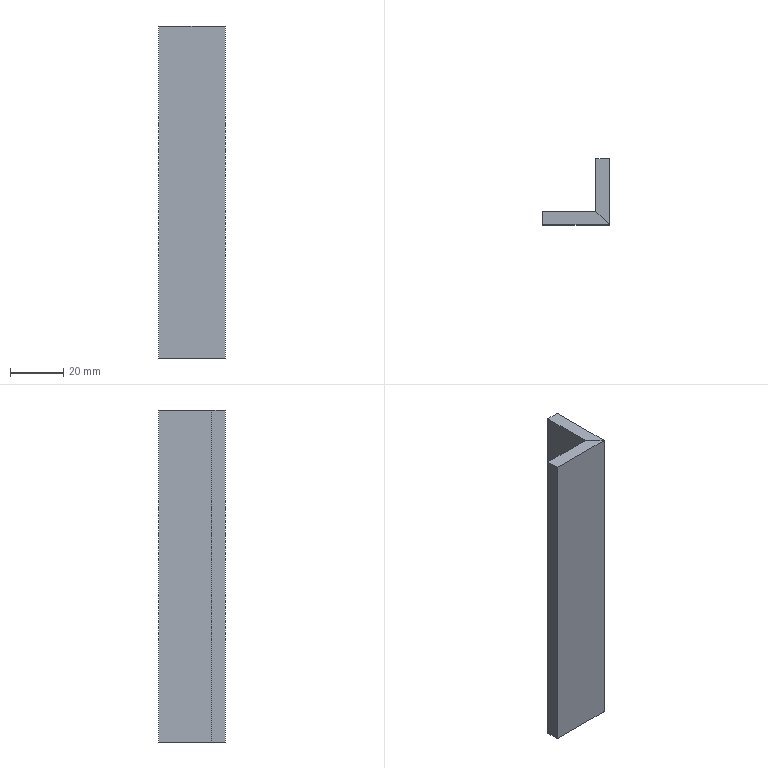Part | NX | features BREP 1 | 1 solid | 10 faces | box 25 x 25 x 125 mm | volume 28125 mm3 | plane 10
STEP:
#1=CARTESIAN_POINT('',(689.674,-673.,218.142));
#2=VERTEX_POINT('',#1);
#3=CARTESIAN_POINT('',(694.674,-673.,218.142));
#4=VERTEX_POINT('',#3);
#5=CARTESIAN_POINT('',(692.174,-673.,218.142));
#6=DIRECTION('',(1.,0.,0.));
#7=VECTOR('',#6,1000.);
#8=LINE('',#5,#7);
#9=EDGE_CURVE('',#2,#4,#8,.T.);
#10=ORIENTED_EDGE('',*,*,#9,.F.);
#11=CARTESIAN_POINT('',(689.674,-693.,218.142));
#12=VERTEX_POINT('',#11);
#13=CARTESIAN_POINT('',(689.674,-683.,218.142));
#14=DIRECTION('',(0.,1.,0.));
#15=VECTOR('',#14,1000.);
#16=LINE('',#13,#15);
#17=EDGE_CURVE('',#12,#2,#16,.T.);
#18=ORIENTED_EDGE('',*,*,#17,.F.);
#19=CARTESIAN_POINT('',(694.674,-698.,218.142));
#20=VERTEX_POINT('',#19);
#21=CARTESIAN_POINT('',(692.174,-695.5,218.142));
#22=DIRECTION('',(-0.7071,0.7071,0.));
#23=VECTOR('',#22,1000.);
#24=LINE('',#21,#23);
#25=EDGE_CURVE('',#20,#12,#24,.T.);
#26=ORIENTED_EDGE('',*,*,#25,.F.);
#27=CARTESIAN_POINT('',(694.674,-685.5,218.142));
#28=DIRECTION('',(0.,1.,0.));
#29=VECTOR('',#28,1000.);
#30=LINE('',#27,#29);
#31=EDGE_CURVE('',#20,#4,#30,.T.);
#32=ORIENTED_EDGE('',*,*,#31,.T.);
#33=EDGE_LOOP('',(#10,#18,#26,#32));
#34=FACE_BOUND('',#33,.T.);
#35=CARTESIAN_POINT('',(694.674,-685.5,218.142));
#36=DIRECTION('',(0.,0.,-1.));
#37=DIRECTION('',(1.,0.,0.));
#38=AXIS2_PLACEMENT_3D('',#35,#36,#37);
#39=PLANE('',#38);
#40=ADVANCED_FACE('',(#34),#39,.F.);
#41=CARTESIAN_POINT('',(689.674,-673.,93.142));
#42=VERTEX_POINT('',#41);
#43=CARTESIAN_POINT('',(694.674,-673.,93.142));
#44=VERTEX_POINT('',#43);
#45=CARTESIAN_POINT('',(692.174,-673.,93.142));
#46=DIRECTION('',(1.,0.,0.));
#47=VECTOR('',#46,1000.);
#48=LINE('',#45,#47);
#49=EDGE_CURVE('',#42,#44,#48,.T.);
#50=ORIENTED_EDGE('',*,*,#49,.F.);
#51=CARTESIAN_POINT('',(689.674,-673.,155.642));
#52=DIRECTION('',(0.,0.,1.));
#53=VECTOR('',#52,1000.);
#54=LINE('',#51,#53);
#55=EDGE_CURVE('',#42,#2,#54,.T.);
#56=ORIENTED_EDGE('',*,*,#55,.T.);
#57=ORIENTED_EDGE('',*,*,#9,.T.);
#58=CARTESIAN_POINT('',(694.674,-673.,155.642));
#59=DIRECTION('',(0.,0.,1.));
#60=VECTOR('',#59,1000.);
#61=LINE('',#58,#60);
#62=EDGE_CURVE('',#44,#4,#61,.T.);
#63=ORIENTED_EDGE('',*,*,#62,.F.);
#64=EDGE_LOOP('',(#50,#56,#57,#63));
#65=FACE_BOUND('',#64,.T.);
#66=CARTESIAN_POINT('',(694.674,-673.,155.642));
#67=DIRECTION('',(0.,1.,0.));
#68=DIRECTION('',(1.,0.,0.));
#69=AXIS2_PLACEMENT_3D('',#66,#67,#68);
#70=PLANE('',#69);
#71=ADVANCED_FACE('',(#65),#70,.T.);
#72=ORIENTED_EDGE('',*,*,#31,.F.);
#73=CARTESIAN_POINT('',(694.674,-698.,93.142));
#74=VERTEX_POINT('',#73);
#75=CARTESIAN_POINT('',(694.674,-698.,155.642));
#76=DIRECTION('',(0.,0.,1.));
#77=VECTOR('',#76,1000.);
#78=LINE('',#75,#77);
#79=EDGE_CURVE('',#74,#20,#78,.T.);
#80=ORIENTED_EDGE('',*,*,#79,.F.);
#81=CARTESIAN_POINT('',(694.674,-685.5,93.142));
#82=DIRECTION('',(0.,-1.,0.));
#83=VECTOR('',#82,1000.);
#84=LINE('',#81,#83);
#85=EDGE_CURVE('',#44,#74,#84,.T.);
#86=ORIENTED_EDGE('',*,*,#85,.F.);
#87=ORIENTED_EDGE('',*,*,#62,.T.);
#88=EDGE_LOOP('',(#72,#80,#86,#87));
#89=FACE_BOUND('',#88,.T.);
#90=CARTESIAN_POINT('',(694.674,-700.,74.));
#91=DIRECTION('',(-1.,0.,0.));
#92=DIRECTION('',(0.,0.,1.));
#93=AXIS2_PLACEMENT_3D('',#90,#91,#92);
#94=PLANE('',#93);
#95=ADVANCED_FACE('',(#89),#94,.F.);
#96=ORIENTED_EDGE('',*,*,#55,.F.);
#97=CARTESIAN_POINT('',(689.674,-693.,93.142));
#98=VERTEX_POINT('',#97);
#99=CARTESIAN_POINT('',(689.674,-683.,93.142));
#100=DIRECTION('',(0.,-1.,0.));
#101=VECTOR('',#100,1000.);
#102=LINE('',#99,#101);
#103=EDGE_CURVE('',#42,#98,#102,.T.);
#104=ORIENTED_EDGE('',*,*,#103,.T.);
#105=CARTESIAN_POINT('',(689.674,-693.,155.642));
#106=DIRECTION('',(0.,0.,1.));
#107=VECTOR('',#106,1000.);
#108=LINE('',#105,#107);
#109=EDGE_CURVE('',#98,#12,#108,.T.);
#110=ORIENTED_EDGE('',*,*,#109,.T.);
#111=ORIENTED_EDGE('',*,*,#17,.T.);
#112=EDGE_LOOP('',(#96,#104,#110,#111));
#113=FACE_BOUND('',#112,.T.);
#114=CARTESIAN_POINT('',(689.674,-700.,74.));
#115=DIRECTION('',(-1.,0.,0.));
#116=DIRECTION('',(0.,0.,1.));
#117=AXIS2_PLACEMENT_3D('',#114,#115,#116);
#118=PLANE('',#117);
#119=ADVANCED_FACE('',(#113),#118,.T.);
#120=CARTESIAN_POINT('',(669.674,-698.,218.142));
#121=VERTEX_POINT('',#120);
#122=CARTESIAN_POINT('',(682.174,-698.,218.142));
#123=DIRECTION('',(-1.,0.,0.));
#124=VECTOR('',#123,1000.);
#125=LINE('',#122,#124);
#126=EDGE_CURVE('',#20,#121,#125,.T.);
#127=ORIENTED_EDGE('',*,*,#126,.F.);
#128=ORIENTED_EDGE('',*,*,#25,.T.);
#129=CARTESIAN_POINT('',(669.674,-693.,218.142));
#130=VERTEX_POINT('',#129);
#131=CARTESIAN_POINT('',(679.674,-693.,218.142));
#132=DIRECTION('',(-1.,0.,0.));
#133=VECTOR('',#132,1000.);
#134=LINE('',#131,#133);
#135=EDGE_CURVE('',#12,#130,#134,.T.);
#136=ORIENTED_EDGE('',*,*,#135,.T.);
#137=CARTESIAN_POINT('',(669.674,-695.5,218.142));
#138=DIRECTION('',(0.,-1.,0.));
#139=VECTOR('',#138,1000.);
#140=LINE('',#137,#139);
#141=EDGE_CURVE('',#130,#121,#140,.T.);
#142=ORIENTED_EDGE('',*,*,#141,.T.);
#143=EDGE_LOOP('',(#127,#128,#136,#142));
#144=FACE_BOUND('',#143,.T.);
#145=CARTESIAN_POINT('',(694.674,-698.,218.142));
#146=DIRECTION('',(0.,0.,1.));
#147=DIRECTION('',(-1.,0.,0.));
#148=AXIS2_PLACEMENT_3D('',#145,#146,#147);
#149=PLANE('',#148);
#150=ADVANCED_FACE('',(#144),#149,.T.);
#151=CARTESIAN_POINT('',(669.674,-698.,93.142));
#152=VERTEX_POINT('',#151);
#153=CARTESIAN_POINT('',(682.174,-698.,93.142));
#154=DIRECTION('',(-1.,0.,0.));
#155=VECTOR('',#154,1000.);
#156=LINE('',#153,#155);
#157=EDGE_CURVE('',#74,#152,#156,.T.);
#158=ORIENTED_EDGE('',*,*,#157,.F.);
#159=ORIENTED_EDGE('',*,*,#79,.T.);
#160=ORIENTED_EDGE('',*,*,#126,.T.);
#161=CARTESIAN_POINT('',(669.674,-698.,155.642));
#162=DIRECTION('',(0.,0.,1.));
#163=VECTOR('',#162,1000.);
#164=LINE('',#161,#163);
#165=EDGE_CURVE('',#152,#121,#164,.T.);
#166=ORIENTED_EDGE('',*,*,#165,.F.);
#167=EDGE_LOOP('',(#158,#159,#160,#166));
#168=FACE_BOUND('',#167,.T.);
#169=CARTESIAN_POINT('',(694.674,-698.,93.142));
#170=DIRECTION('',(0.,-1.,0.));
#171=DIRECTION('',(0.,0.,1.));
#172=AXIS2_PLACEMENT_3D('',#169,#170,#171);
#173=PLANE('',#172);
#174=ADVANCED_FACE('',(#168),#173,.T.);
#175=ORIENTED_EDGE('',*,*,#85,.T.);
#176=CARTESIAN_POINT('',(692.174,-695.5,93.142));
#177=DIRECTION('',(-0.7071,0.7071,0.));
#178=VECTOR('',#177,1000.);
#179=LINE('',#176,#178);
#180=EDGE_CURVE('',#74,#98,#179,.T.);
#181=ORIENTED_EDGE('',*,*,#180,.T.);
#182=ORIENTED_EDGE('',*,*,#103,.F.);
#183=ORIENTED_EDGE('',*,*,#49,.T.);
#184=EDGE_LOOP('',(#175,#181,#182,#183));
#185=FACE_BOUND('',#184,.T.);
#186=CARTESIAN_POINT('',(694.674,-685.5,93.142));
#187=DIRECTION('',(0.,0.,-1.));
#188=DIRECTION('',(1.,0.,0.));
#189=AXIS2_PLACEMENT_3D('',#186,#187,#188);
#190=PLANE('',#189);
#191=ADVANCED_FACE('',(#185),#190,.T.);
#192=CARTESIAN_POINT('',(669.674,-693.,93.142));
#193=VERTEX_POINT('',#192);
#194=CARTESIAN_POINT('',(669.674,-693.,155.642));
#195=DIRECTION('',(0.,0.,1.));
#196=VECTOR('',#195,1000.);
#197=LINE('',#194,#196);
#198=EDGE_CURVE('',#193,#130,#197,.T.);
#199=ORIENTED_EDGE('',*,*,#198,.T.);
#200=ORIENTED_EDGE('',*,*,#135,.F.);
#201=ORIENTED_EDGE('',*,*,#109,.F.);
#202=CARTESIAN_POINT('',(679.674,-693.,93.142));
#203=DIRECTION('',(-1.,0.,0.));
#204=VECTOR('',#203,1000.);
#205=LINE('',#202,#204);
#206=EDGE_CURVE('',#98,#193,#205,.T.);
#207=ORIENTED_EDGE('',*,*,#206,.T.);
#208=EDGE_LOOP('',(#199,#200,#201,#207));
#209=FACE_BOUND('',#208,.T.);
#210=CARTESIAN_POINT('',(689.674,-693.,93.142));
#211=DIRECTION('',(0.,-1.,0.));
#212=DIRECTION('',(0.,0.,1.));
#213=AXIS2_PLACEMENT_3D('',#210,#211,#212);
#214=PLANE('',#213);
#215=ADVANCED_FACE('',(#209),#214,.F.);
#216=ORIENTED_EDGE('',*,*,#165,.T.);
#217=ORIENTED_EDGE('',*,*,#141,.F.);
#218=ORIENTED_EDGE('',*,*,#198,.F.);
#219=CARTESIAN_POINT('',(669.674,-695.5,93.142));
#220=DIRECTION('',(0.,-1.,0.));
#221=VECTOR('',#220,1000.);
#222=LINE('',#219,#221);
#223=EDGE_CURVE('',#193,#152,#222,.T.);
#224=ORIENTED_EDGE('',*,*,#223,.T.);
#225=EDGE_LOOP('',(#216,#217,#218,#224));
#226=FACE_BOUND('',#225,.T.);
#227=CARTESIAN_POINT('',(669.674,-698.,93.142));
#228=DIRECTION('',(1.,0.,0.));
#229=DIRECTION('',(0.,0.,1.));
#230=AXIS2_PLACEMENT_3D('',#227,#228,#229);
#231=PLANE('',#230);
#232=ADVANCED_FACE('',(#226),#231,.F.);
#233=ORIENTED_EDGE('',*,*,#223,.F.);
#234=ORIENTED_EDGE('',*,*,#206,.F.);
#235=ORIENTED_EDGE('',*,*,#180,.F.);
#236=ORIENTED_EDGE('',*,*,#157,.T.);
#237=EDGE_LOOP('',(#233,#234,#235,#236));
#238=FACE_BOUND('',#237,.T.);
#239=CARTESIAN_POINT('',(694.674,-698.,93.142));
#240=DIRECTION('',(0.,0.,1.));
#241=DIRECTION('',(-1.,0.,0.));
#242=AXIS2_PLACEMENT_3D('',#239,#240,#241);
#243=PLANE('',#242);
#244=ADVANCED_FACE('',(#238),#243,.F.);
#245=CLOSED_SHELL('',(#40,#71,#95,#119,#150,#174,#191,#215,#232,#244));
#246=MANIFOLD_SOLID_BREP('',#245);
#247=(LENGTH_UNIT()NAMED_UNIT(*)SI_UNIT(.MILLI.,.METRE.));
#248=UNCERTAINTY_MEASURE_WITH_UNIT(LENGTH_MEASURE(0.00001),#247,'','');
#249=(NAMED_UNIT(*)PLANE_ANGLE_UNIT()SI_UNIT($,.RADIAN.));
#250=(NAMED_UNIT(*)SI_UNIT($,.STERADIAN.)SOLID_ANGLE_UNIT());
#251=(GEOMETRIC_REPRESENTATION_CONTEXT(3)GLOBAL_UNCERTAINTY_ASSIGNED_CONTEXT((#248))GLOBAL_UNIT_ASSIGNED_CONTEXT((#247,#249,#250))REPRESENTATION_CONTEXT('',''));
#252=ADVANCED_BREP_SHAPE_REPRESENTATION('',(#246),#251);